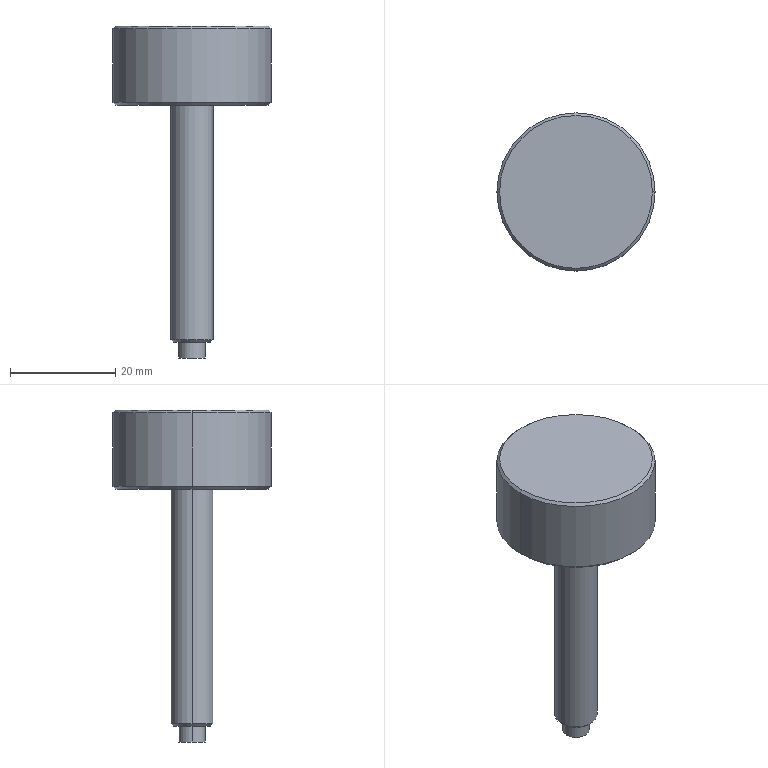Part | SolidWorks | features ICE 3, Chamfer 1, Extrusion 1 | 2 solids | 20 faces | box 30 x 30 x 63 mm | volume 12897 mm3 | cylinder 8 | cone 6 | plane 6 | commonest cylinder face diameters 5 x4 8 x2 30 x2
STEP:
#1=CARTESIAN_POINT('',(14.5,0.,60.));
#2=VERTEX_POINT('',#1);
#3=CARTESIAN_POINT('',(-14.5,0.,60.));
#4=VERTEX_POINT('',#3);
#5=CARTESIAN_POINT('',(0.,0.,60.));
#6=DIRECTION('',(0.,0.,1.));
#7=DIRECTION('',(1.,0.,0.));
#8=AXIS2_PLACEMENT_3D('',#5,#6,#7);
#9=CIRCLE('',#8,14.5);
#10=EDGE_CURVE('',#2,#4,#9,.T.);
#11=ORIENTED_EDGE('',*,*,#10,.F.);
#12=CARTESIAN_POINT('',(15.,0.,59.5));
#13=VERTEX_POINT('',#12);
#14=CARTESIAN_POINT('',(14.5,0.,60.));
#15=DIRECTION('',(0.7071,0.,-0.7071));
#16=VECTOR('',#15,1000.);
#17=LINE('',#14,#16);
#18=EDGE_CURVE('',#2,#13,#17,.T.);
#19=ORIENTED_EDGE('',*,*,#18,.T.);
#20=CARTESIAN_POINT('',(-15.,0.,59.5));
#21=VERTEX_POINT('',#20);
#22=CARTESIAN_POINT('',(0.,0.,59.5));
#23=DIRECTION('',(0.,0.,-1.));
#24=DIRECTION('',(1.,0.,0.));
#25=AXIS2_PLACEMENT_3D('',#22,#23,#24);
#26=CIRCLE('',#25,15.);
#27=EDGE_CURVE('',#21,#13,#26,.T.);
#28=ORIENTED_EDGE('',*,*,#27,.F.);
#29=CARTESIAN_POINT('',(-14.5,0.,60.));
#30=DIRECTION('',(-0.7071,0.,-0.7071));
#31=VECTOR('',#30,1000.);
#32=LINE('',#29,#31);
#33=EDGE_CURVE('',#4,#21,#32,.T.);
#34=ORIENTED_EDGE('',*,*,#33,.F.);
#35=EDGE_LOOP('',(#11,#19,#28,#34));
#36=FACE_OUTER_BOUND('',#35,.T.);
#37=CARTESIAN_POINT('',(0.,0.,60.));
#38=DIRECTION('',(0.,0.,-1.));
#39=DIRECTION('',(-1.,0.,0.));
#40=AXIS2_PLACEMENT_3D('',#37,#38,#39);
#41=CONICAL_SURFACE('',#40,14.5,0.7854);
#42=ADVANCED_FACE('',(#36),#41,.T.);
#43=CARTESIAN_POINT('',(-14.5,0.,45.));
#44=VERTEX_POINT('',#43);
#45=CARTESIAN_POINT('',(14.5,0.,45.));
#46=VERTEX_POINT('',#45);
#47=CARTESIAN_POINT('',(0.,0.,45.));
#48=DIRECTION('',(0.,0.,-1.));
#49=DIRECTION('',(1.,0.,0.));
#50=AXIS2_PLACEMENT_3D('',#47,#48,#49);
#51=CIRCLE('',#50,14.5);
#52=EDGE_CURVE('',#44,#46,#51,.T.);
#53=ORIENTED_EDGE('',*,*,#52,.F.);
#54=CARTESIAN_POINT('',(-15.,0.,45.5));
#55=VERTEX_POINT('',#54);
#56=CARTESIAN_POINT('',(-15.,0.,45.5));
#57=DIRECTION('',(-0.7071,0.,0.7071));
#58=VECTOR('',#57,1000.);
#59=LINE('',#56,#58);
#60=EDGE_CURVE('',#44,#55,#59,.T.);
#61=ORIENTED_EDGE('',*,*,#60,.T.);
#62=CARTESIAN_POINT('',(15.,0.,45.5));
#63=VERTEX_POINT('',#62);
#64=CARTESIAN_POINT('',(0.,0.,45.5));
#65=DIRECTION('',(0.,0.,1.));
#66=DIRECTION('',(1.,0.,0.));
#67=AXIS2_PLACEMENT_3D('',#64,#65,#66);
#68=CIRCLE('',#67,15.);
#69=EDGE_CURVE('',#63,#55,#68,.T.);
#70=ORIENTED_EDGE('',*,*,#69,.F.);
#71=CARTESIAN_POINT('',(15.,0.,45.5));
#72=DIRECTION('',(0.7071,0.,0.7071));
#73=VECTOR('',#72,1000.);
#74=LINE('',#71,#73);
#75=EDGE_CURVE('',#46,#63,#74,.T.);
#76=ORIENTED_EDGE('',*,*,#75,.F.);
#77=EDGE_LOOP('',(#53,#61,#70,#76));
#78=FACE_OUTER_BOUND('',#77,.T.);
#79=CARTESIAN_POINT('',(0.,0.,45.5));
#80=DIRECTION('',(0.,0.,1.));
#81=DIRECTION('',(1.,0.,0.));
#82=AXIS2_PLACEMENT_3D('',#79,#80,#81);
#83=CONICAL_SURFACE('',#82,15.,0.7854);
#84=ADVANCED_FACE('',(#78),#83,.T.);
#85=CARTESIAN_POINT('',(-3.5,0.,0.));
#86=VERTEX_POINT('',#85);
#87=CARTESIAN_POINT('',(3.5,0.,0.));
#88=VERTEX_POINT('',#87);
#89=CARTESIAN_POINT('',(0.,0.,0.));
#90=DIRECTION('',(0.,0.,-1.));
#91=DIRECTION('',(1.,0.,0.));
#92=AXIS2_PLACEMENT_3D('',#89,#90,#91);
#93=CIRCLE('',#92,3.5);
#94=EDGE_CURVE('',#86,#88,#93,.T.);
#95=ORIENTED_EDGE('',*,*,#94,.F.);
#96=CARTESIAN_POINT('',(-4.,0.,0.5));
#97=VERTEX_POINT('',#96);
#98=CARTESIAN_POINT('',(-4.,0.,0.5));
#99=DIRECTION('',(-0.7071,0.,0.7071));
#100=VECTOR('',#99,1000.);
#101=LINE('',#98,#100);
#102=EDGE_CURVE('',#86,#97,#101,.T.);
#103=ORIENTED_EDGE('',*,*,#102,.T.);
#104=CARTESIAN_POINT('',(4.,0.,0.5));
#105=VERTEX_POINT('',#104);
#106=CARTESIAN_POINT('',(0.,0.,0.5));
#107=DIRECTION('',(0.,0.,1.));
#108=DIRECTION('',(1.,0.,0.));
#109=AXIS2_PLACEMENT_3D('',#106,#107,#108);
#110=CIRCLE('',#109,4.);
#111=EDGE_CURVE('',#105,#97,#110,.T.);
#112=ORIENTED_EDGE('',*,*,#111,.F.);
#113=CARTESIAN_POINT('',(4.,0.,0.5));
#114=DIRECTION('',(0.7071,0.,0.7071));
#115=VECTOR('',#114,1000.);
#116=LINE('',#113,#115);
#117=EDGE_CURVE('',#88,#105,#116,.T.);
#118=ORIENTED_EDGE('',*,*,#117,.F.);
#119=EDGE_LOOP('',(#95,#103,#112,#118));
#120=FACE_OUTER_BOUND('',#119,.T.);
#121=CARTESIAN_POINT('',(0.,0.,0.5));
#122=DIRECTION('',(0.,0.,1.));
#123=DIRECTION('',(1.,0.,0.));
#124=AXIS2_PLACEMENT_3D('',#121,#122,#123);
#125=CONICAL_SURFACE('',#124,4.,0.7854);
#126=ADVANCED_FACE('',(#120),#125,.T.);
#127=CARTESIAN_POINT('',(2.5,0.,4.));
#128=VERTEX_POINT('',#127);
#129=CARTESIAN_POINT('',(-2.5,0.,4.));
#130=VERTEX_POINT('',#129);
#131=CARTESIAN_POINT('',(0.,0.,4.));
#132=DIRECTION('',(0.,0.,-1.));
#133=DIRECTION('',(-1.,0.,0.));
#134=AXIS2_PLACEMENT_3D('',#131,#132,#133);
#135=CIRCLE('',#134,2.5);
#136=EDGE_CURVE('',#128,#130,#135,.T.);
#137=ORIENTED_EDGE('',*,*,#136,.F.);
#138=CARTESIAN_POINT('',(2.5,0.,0.));
#139=VERTEX_POINT('',#138);
#140=CARTESIAN_POINT('',(2.5,0.,4.));
#141=DIRECTION('',(0.,0.,-1.));
#142=VECTOR('',#141,1000.);
#143=LINE('',#140,#142);
#144=EDGE_CURVE('',#128,#139,#143,.T.);
#145=ORIENTED_EDGE('',*,*,#144,.T.);
#146=CARTESIAN_POINT('',(-2.5,0.,0.));
#147=VERTEX_POINT('',#146);
#148=CARTESIAN_POINT('',(0.,0.,0.));
#149=DIRECTION('',(0.,0.,-1.));
#150=DIRECTION('',(-1.,0.,0.));
#151=AXIS2_PLACEMENT_3D('',#148,#149,#150);
#152=CIRCLE('',#151,2.5);
#153=EDGE_CURVE('',#139,#147,#152,.T.);
#154=ORIENTED_EDGE('',*,*,#153,.T.);
#155=CARTESIAN_POINT('',(-2.5,0.,4.));
#156=DIRECTION('',(0.,0.,-1.));
#157=VECTOR('',#156,1000.);
#158=LINE('',#155,#157);
#159=EDGE_CURVE('',#130,#147,#158,.T.);
#160=ORIENTED_EDGE('',*,*,#159,.F.);
#161=EDGE_LOOP('',(#137,#145,#154,#160));
#162=FACE_OUTER_BOUND('',#161,.T.);
#163=CARTESIAN_POINT('',(0.,0.,4.));
#164=DIRECTION('',(0.,0.,-1.));
#165=DIRECTION('',(-1.,0.,0.));
#166=AXIS2_PLACEMENT_3D('',#163,#164,#165);
#167=CYLINDRICAL_SURFACE('',#166,2.5);
#168=ADVANCED_FACE('',(#162),#167,.F.);
#169=ORIENTED_EDGE('',*,*,#27,.T.);
#170=CARTESIAN_POINT('',(15.,0.,60.));
#171=DIRECTION('',(0.,0.,-1.));
#172=VECTOR('',#171,1000.);
#173=LINE('',#170,#172);
#174=EDGE_CURVE('',#13,#63,#173,.T.);
#175=ORIENTED_EDGE('',*,*,#174,.T.);
#176=ORIENTED_EDGE('',*,*,#69,.T.);
#177=CARTESIAN_POINT('',(-15.,0.,60.));
#178=DIRECTION('',(0.,0.,-1.));
#179=VECTOR('',#178,1000.);
#180=LINE('',#177,#179);
#181=EDGE_CURVE('',#21,#55,#180,.T.);
#182=ORIENTED_EDGE('',*,*,#181,.F.);
#183=EDGE_LOOP('',(#169,#175,#176,#182));
#184=FACE_OUTER_BOUND('',#183,.T.);
#185=CARTESIAN_POINT('',(0.,0.,60.));
#186=DIRECTION('',(0.,0.,-1.));
#187=DIRECTION('',(-1.,0.,0.));
#188=AXIS2_PLACEMENT_3D('',#185,#186,#187);
#189=CYLINDRICAL_SURFACE('',#188,15.);
#190=ADVANCED_FACE('',(#184),#189,.T.);
#191=CARTESIAN_POINT('',(4.,0.,45.));
#192=VERTEX_POINT('',#191);
#193=CARTESIAN_POINT('',(-4.,0.,45.));
#194=VERTEX_POINT('',#193);
#195=CARTESIAN_POINT('',(0.,0.,45.));
#196=DIRECTION('',(0.,0.,1.));
#197=DIRECTION('',(1.,0.,0.));
#198=AXIS2_PLACEMENT_3D('',#195,#196,#197);
#199=CIRCLE('',#198,4.);
#200=EDGE_CURVE('',#192,#194,#199,.T.);
#201=ORIENTED_EDGE('',*,*,#200,.F.);
#202=CARTESIAN_POINT('',(4.,0.,45.));
#203=DIRECTION('',(0.,0.,-1.));
#204=VECTOR('',#203,1000.);
#205=LINE('',#202,#204);
#206=EDGE_CURVE('',#192,#105,#205,.T.);
#207=ORIENTED_EDGE('',*,*,#206,.T.);
#208=ORIENTED_EDGE('',*,*,#111,.T.);
#209=CARTESIAN_POINT('',(-4.,0.,45.));
#210=DIRECTION('',(0.,0.,-1.));
#211=VECTOR('',#210,1000.);
#212=LINE('',#209,#211);
#213=EDGE_CURVE('',#194,#97,#212,.T.);
#214=ORIENTED_EDGE('',*,*,#213,.F.);
#215=EDGE_LOOP('',(#201,#207,#208,#214));
#216=FACE_OUTER_BOUND('',#215,.T.);
#217=CARTESIAN_POINT('',(0.,0.,45.));
#218=DIRECTION('',(0.,0.,-1.));
#219=DIRECTION('',(-1.,0.,0.));
#220=AXIS2_PLACEMENT_3D('',#217,#218,#219);
#221=CYLINDRICAL_SURFACE('',#220,4.);
#222=ADVANCED_FACE('',(#216),#221,.T.);
#223=ORIENTED_EDGE('',*,*,#206,.F.);
#224=CARTESIAN_POINT('',(0.,0.,45.));
#225=DIRECTION('',(0.,0.,1.));
#226=DIRECTION('',(1.,0.,0.));
#227=AXIS2_PLACEMENT_3D('',#224,#225,#226);
#228=CIRCLE('',#227,4.);
#229=EDGE_CURVE('',#194,#192,#228,.T.);
#230=ORIENTED_EDGE('',*,*,#229,.F.);
#231=ORIENTED_EDGE('',*,*,#213,.T.);
#232=CARTESIAN_POINT('',(0.,0.,0.5));
#233=DIRECTION('',(0.,0.,1.));
#234=DIRECTION('',(1.,0.,0.));
#235=AXIS2_PLACEMENT_3D('',#232,#233,#234);
#236=CIRCLE('',#235,4.);
#237=EDGE_CURVE('',#97,#105,#236,.T.);
#238=ORIENTED_EDGE('',*,*,#237,.T.);
#239=EDGE_LOOP('',(#223,#230,#231,#238));
#240=FACE_OUTER_BOUND('',#239,.T.);
#241=CARTESIAN_POINT('',(0.,0.,45.));
#242=DIRECTION('',(0.,0.,-1.));
#243=DIRECTION('',(-1.,0.,0.));
#244=AXIS2_PLACEMENT_3D('',#241,#242,#243);
#245=CYLINDRICAL_SURFACE('',#244,4.);
#246=ADVANCED_FACE('',(#240),#245,.T.);
#247=CARTESIAN_POINT('',(0.,0.,0.));
#248=DIRECTION('',(0.,0.,-1.));
#249=DIRECTION('',(1.,0.,0.));
#250=AXIS2_PLACEMENT_3D('',#247,#248,#249);
#251=CIRCLE('',#250,3.5);
#252=EDGE_CURVE('',#88,#86,#251,.T.);
#253=ORIENTED_EDGE('',*,*,#252,.T.);
#254=ORIENTED_EDGE('',*,*,#94,.T.);
#255=EDGE_LOOP('',(#253,#254));
#256=FACE_OUTER_BOUND('',#255,.T.);
#257=CARTESIAN_POINT('',(0.,0.,0.));
#258=DIRECTION('',(0.,0.,-1.));
#259=DIRECTION('',(-1.,0.,0.));
#260=AXIS2_PLACEMENT_3D('',#257,#258,#259);
#261=CIRCLE('',#260,2.5);
#262=EDGE_CURVE('',#147,#139,#261,.T.);
#263=ORIENTED_EDGE('',*,*,#262,.F.);
#264=ORIENTED_EDGE('',*,*,#153,.F.);
#265=EDGE_LOOP('',(#263,#264));
#266=FACE_BOUND('',#265,.T.);
#267=CARTESIAN_POINT('',(0.,0.,0.));
#268=DIRECTION('',(0.,0.,1.));
#269=DIRECTION('',(1.,0.,0.));
#270=AXIS2_PLACEMENT_3D('',#267,#268,#269);
#271=PLANE('',#270);
#272=ADVANCED_FACE('',(#256,#266),#271,.F.);
#273=CARTESIAN_POINT('',(0.,0.,45.));
#274=DIRECTION('',(0.,0.,-1.));
#275=DIRECTION('',(1.,0.,0.));
#276=AXIS2_PLACEMENT_3D('',#273,#274,#275);
#277=CIRCLE('',#276,14.5);
#278=EDGE_CURVE('',#46,#44,#277,.T.);
#279=ORIENTED_EDGE('',*,*,#278,.T.);
#280=ORIENTED_EDGE('',*,*,#52,.T.);
#281=EDGE_LOOP('',(#279,#280));
#282=FACE_OUTER_BOUND('',#281,.T.);
#283=ORIENTED_EDGE('',*,*,#229,.T.);
#284=ORIENTED_EDGE('',*,*,#200,.T.);
#285=EDGE_LOOP('',(#283,#284));
#286=FACE_BOUND('',#285,.T.);
#287=CARTESIAN_POINT('',(0.,0.,45.));
#288=DIRECTION('',(0.,0.,1.));
#289=DIRECTION('',(1.,0.,0.));
#290=AXIS2_PLACEMENT_3D('',#287,#288,#289);
#291=PLANE('',#290);
#292=ADVANCED_FACE('',(#282,#286),#291,.F.);
#293=ORIENTED_EDGE('',*,*,#174,.F.);
#294=CARTESIAN_POINT('',(0.,0.,59.5));
#295=DIRECTION('',(0.,0.,-1.));
#296=DIRECTION('',(1.,0.,0.));
#297=AXIS2_PLACEMENT_3D('',#294,#295,#296);
#298=CIRCLE('',#297,15.);
#299=EDGE_CURVE('',#13,#21,#298,.T.);
#300=ORIENTED_EDGE('',*,*,#299,.T.);
#301=ORIENTED_EDGE('',*,*,#181,.T.);
#302=CARTESIAN_POINT('',(0.,0.,45.5));
#303=DIRECTION('',(0.,0.,1.));
#304=DIRECTION('',(1.,0.,0.));
#305=AXIS2_PLACEMENT_3D('',#302,#303,#304);
#306=CIRCLE('',#305,15.);
#307=EDGE_CURVE('',#55,#63,#306,.T.);
#308=ORIENTED_EDGE('',*,*,#307,.T.);
#309=EDGE_LOOP('',(#293,#300,#301,#308));
#310=FACE_OUTER_BOUND('',#309,.T.);
#311=CARTESIAN_POINT('',(0.,0.,60.));
#312=DIRECTION('',(0.,0.,-1.));
#313=DIRECTION('',(-1.,0.,0.));
#314=AXIS2_PLACEMENT_3D('',#311,#312,#313);
#315=CYLINDRICAL_SURFACE('',#314,15.);
#316=ADVANCED_FACE('',(#310),#315,.T.);
#317=CARTESIAN_POINT('',(0.,0.,60.));
#318=DIRECTION('',(0.,0.,1.));
#319=DIRECTION('',(1.,0.,0.));
#320=AXIS2_PLACEMENT_3D('',#317,#318,#319);
#321=CIRCLE('',#320,14.5);
#322=EDGE_CURVE('',#4,#2,#321,.T.);
#323=ORIENTED_EDGE('',*,*,#322,.T.);
#324=ORIENTED_EDGE('',*,*,#10,.T.);
#325=EDGE_LOOP('',(#323,#324));
#326=FACE_OUTER_BOUND('',#325,.T.);
#327=CARTESIAN_POINT('',(0.,0.,60.));
#328=DIRECTION('',(0.,0.,1.));
#329=DIRECTION('',(1.,0.,0.));
#330=AXIS2_PLACEMENT_3D('',#327,#328,#329);
#331=PLANE('',#330);
#332=ADVANCED_FACE('',(#326),#331,.T.);
#333=ORIENTED_EDGE('',*,*,#144,.F.);
#334=CARTESIAN_POINT('',(0.,0.,4.));
#335=DIRECTION('',(0.,0.,-1.));
#336=DIRECTION('',(-1.,0.,0.));
#337=AXIS2_PLACEMENT_3D('',#334,#335,#336);
#338=CIRCLE('',#337,2.5);
#339=EDGE_CURVE('',#130,#128,#338,.T.);
#340=ORIENTED_EDGE('',*,*,#339,.F.);
#341=ORIENTED_EDGE('',*,*,#159,.T.);
#342=ORIENTED_EDGE('',*,*,#262,.T.);
#343=EDGE_LOOP('',(#333,#340,#341,#342));
#344=FACE_OUTER_BOUND('',#343,.T.);
#345=CARTESIAN_POINT('',(0.,0.,4.));
#346=DIRECTION('',(0.,0.,-1.));
#347=DIRECTION('',(-1.,0.,0.));
#348=AXIS2_PLACEMENT_3D('',#345,#346,#347);
#349=CYLINDRICAL_SURFACE('',#348,2.5);
#350=ADVANCED_FACE('',(#344),#349,.F.);
#351=ORIENTED_EDGE('',*,*,#339,.T.);
#352=ORIENTED_EDGE('',*,*,#136,.T.);
#353=EDGE_LOOP('',(#351,#352));
#354=FACE_OUTER_BOUND('',#353,.T.);
#355=CARTESIAN_POINT('',(0.,0.,4.));
#356=DIRECTION('',(0.,0.,-1.));
#357=DIRECTION('',(-1.,0.,0.));
#358=AXIS2_PLACEMENT_3D('',#355,#356,#357);
#359=PLANE('',#358);
#360=ADVANCED_FACE('',(#354),#359,.T.);
#361=ORIENTED_EDGE('',*,*,#102,.F.);
#362=ORIENTED_EDGE('',*,*,#252,.F.);
#363=ORIENTED_EDGE('',*,*,#117,.T.);
#364=ORIENTED_EDGE('',*,*,#237,.F.);
#365=EDGE_LOOP('',(#361,#362,#363,#364));
#366=FACE_OUTER_BOUND('',#365,.T.);
#367=CARTESIAN_POINT('',(0.,0.,0.5));
#368=DIRECTION('',(0.,0.,1.));
#369=DIRECTION('',(1.,0.,0.));
#370=AXIS2_PLACEMENT_3D('',#367,#368,#369);
#371=CONICAL_SURFACE('',#370,4.,0.7854);
#372=ADVANCED_FACE('',(#366),#371,.T.);
#373=ORIENTED_EDGE('',*,*,#60,.F.);
#374=ORIENTED_EDGE('',*,*,#278,.F.);
#375=ORIENTED_EDGE('',*,*,#75,.T.);
#376=ORIENTED_EDGE('',*,*,#307,.F.);
#377=EDGE_LOOP('',(#373,#374,#375,#376));
#378=FACE_OUTER_BOUND('',#377,.T.);
#379=CARTESIAN_POINT('',(0.,0.,45.5));
#380=DIRECTION('',(0.,0.,1.));
#381=DIRECTION('',(1.,0.,0.));
#382=AXIS2_PLACEMENT_3D('',#379,#380,#381);
#383=CONICAL_SURFACE('',#382,15.,0.7854);
#384=ADVANCED_FACE('',(#378),#383,.T.);
#385=ORIENTED_EDGE('',*,*,#18,.F.);
#386=ORIENTED_EDGE('',*,*,#322,.F.);
#387=ORIENTED_EDGE('',*,*,#33,.T.);
#388=ORIENTED_EDGE('',*,*,#299,.F.);
#389=EDGE_LOOP('',(#385,#386,#387,#388));
#390=FACE_OUTER_BOUND('',#389,.T.);
#391=CARTESIAN_POINT('',(0.,0.,60.));
#392=DIRECTION('',(0.,0.,-1.));
#393=DIRECTION('',(-1.,0.,0.));
#394=AXIS2_PLACEMENT_3D('',#391,#392,#393);
#395=CONICAL_SURFACE('',#394,14.5,0.7854);
#396=ADVANCED_FACE('',(#390),#395,.T.);
#397=CLOSED_SHELL('',(#42,#84,#126,#168,#190,#222,#246,#272,#292,#316,#332,#350,#360,#372,#384,#396));
#398=MANIFOLD_SOLID_BREP('',#397);
#399=CARTESIAN_POINT('',(-2.5,0.,-3.));
#400=VERTEX_POINT('',#399);
#401=CARTESIAN_POINT('',(2.5,0.,-3.));
#402=VERTEX_POINT('',#401);
#403=CARTESIAN_POINT('',(0.,0.,-3.));
#404=DIRECTION('',(0.,0.,-1.));
#405=DIRECTION('',(-1.,0.,0.));
#406=AXIS2_PLACEMENT_3D('',#403,#404,#405);
#407=CIRCLE('',#406,2.5);
#408=EDGE_CURVE('',#400,#402,#407,.T.);
#409=ORIENTED_EDGE('',*,*,#408,.F.);
#410=CARTESIAN_POINT('',(-2.5,0.,4.));
#411=VERTEX_POINT('',#410);
#412=CARTESIAN_POINT('',(-2.5,0.,-3.));
#413=DIRECTION('',(0.,0.,1.));
#414=VECTOR('',#413,1000.);
#415=LINE('',#412,#414);
#416=EDGE_CURVE('',#400,#411,#415,.T.);
#417=ORIENTED_EDGE('',*,*,#416,.T.);
#418=CARTESIAN_POINT('',(2.5,0.,4.));
#419=VERTEX_POINT('',#418);
#420=CARTESIAN_POINT('',(0.,0.,4.));
#421=DIRECTION('',(0.,0.,-1.));
#422=DIRECTION('',(-1.,0.,0.));
#423=AXIS2_PLACEMENT_3D('',#420,#421,#422);
#424=CIRCLE('',#423,2.5);
#425=EDGE_CURVE('',#411,#419,#424,.T.);
#426=ORIENTED_EDGE('',*,*,#425,.T.);
#427=CARTESIAN_POINT('',(2.5,0.,-3.));
#428=DIRECTION('',(0.,0.,1.));
#429=VECTOR('',#428,1000.);
#430=LINE('',#427,#429);
#431=EDGE_CURVE('',#402,#419,#430,.T.);
#432=ORIENTED_EDGE('',*,*,#431,.F.);
#433=EDGE_LOOP('',(#409,#417,#426,#432));
#434=FACE_OUTER_BOUND('',#433,.T.);
#435=CARTESIAN_POINT('',(0.,0.,-3.));
#436=DIRECTION('',(0.,0.,1.));
#437=DIRECTION('',(1.,0.,0.));
#438=AXIS2_PLACEMENT_3D('',#435,#436,#437);
#439=CYLINDRICAL_SURFACE('',#438,2.5);
#440=ADVANCED_FACE('',(#434),#439,.T.);
#441=ORIENTED_EDGE('',*,*,#416,.F.);
#442=CARTESIAN_POINT('',(0.,0.,-3.));
#443=DIRECTION('',(0.,0.,-1.));
#444=DIRECTION('',(-1.,0.,0.));
#445=AXIS2_PLACEMENT_3D('',#442,#443,#444);
#446=CIRCLE('',#445,2.5);
#447=EDGE_CURVE('',#402,#400,#446,.T.);
#448=ORIENTED_EDGE('',*,*,#447,.F.);
#449=ORIENTED_EDGE('',*,*,#431,.T.);
#450=CARTESIAN_POINT('',(0.,0.,4.));
#451=DIRECTION('',(0.,0.,-1.));
#452=DIRECTION('',(-1.,0.,0.));
#453=AXIS2_PLACEMENT_3D('',#450,#451,#452);
#454=CIRCLE('',#453,2.5);
#455=EDGE_CURVE('',#419,#411,#454,.T.);
#456=ORIENTED_EDGE('',*,*,#455,.T.);
#457=EDGE_LOOP('',(#441,#448,#449,#456));
#458=FACE_OUTER_BOUND('',#457,.T.);
#459=CARTESIAN_POINT('',(0.,0.,-3.));
#460=DIRECTION('',(0.,0.,1.));
#461=DIRECTION('',(1.,0.,0.));
#462=AXIS2_PLACEMENT_3D('',#459,#460,#461);
#463=CYLINDRICAL_SURFACE('',#462,2.5);
#464=ADVANCED_FACE('',(#458),#463,.T.);
#465=ORIENTED_EDGE('',*,*,#447,.T.);
#466=ORIENTED_EDGE('',*,*,#408,.T.);
#467=EDGE_LOOP('',(#465,#466));
#468=FACE_OUTER_BOUND('',#467,.T.);
#469=CARTESIAN_POINT('',(0.,0.,-3.));
#470=DIRECTION('',(0.,0.,-1.));
#471=DIRECTION('',(-1.,0.,0.));
#472=AXIS2_PLACEMENT_3D('',#469,#470,#471);
#473=PLANE('',#472);
#474=ADVANCED_FACE('',(#468),#473,.T.);
#475=ORIENTED_EDGE('',*,*,#455,.F.);
#476=ORIENTED_EDGE('',*,*,#425,.F.);
#477=EDGE_LOOP('',(#475,#476));
#478=FACE_OUTER_BOUND('',#477,.T.);
#479=CARTESIAN_POINT('',(0.,0.,4.));
#480=DIRECTION('',(0.,0.,-1.));
#481=DIRECTION('',(-1.,0.,0.));
#482=AXIS2_PLACEMENT_3D('',#479,#480,#481);
#483=PLANE('',#482);
#484=ADVANCED_FACE('',(#478),#483,.F.);
#485=CLOSED_SHELL('',(#440,#464,#474,#484));
#486=MANIFOLD_SOLID_BREP('',#485);
#487=CARTESIAN_POINT('',(0.,0.,0.));
#488=DIRECTION('',(0.,0.,1.));
#489=DIRECTION('',(1.,0.,0.));
#490=AXIS2_PLACEMENT_3D('',#487,#488,#489);
#491=(LENGTH_UNIT()NAMED_UNIT(*)SI_UNIT(.MILLI.,.METRE.));
#492=UNCERTAINTY_MEASURE_WITH_UNIT(LENGTH_MEASURE(0.00001),#491,'','');
#493=(NAMED_UNIT(*)PLANE_ANGLE_UNIT()SI_UNIT($,.RADIAN.));
#494=(NAMED_UNIT(*)SI_UNIT($,.STERADIAN.)SOLID_ANGLE_UNIT());
#495=(GEOMETRIC_REPRESENTATION_CONTEXT(3)GLOBAL_UNCERTAINTY_ASSIGNED_CONTEXT((#492))GLOBAL_UNIT_ASSIGNED_CONTEXT((#491,#493,#494))REPRESENTATION_CONTEXT('',''));
#496=ADVANCED_BREP_SHAPE_REPRESENTATION('',(#398,#486,#490),#495);